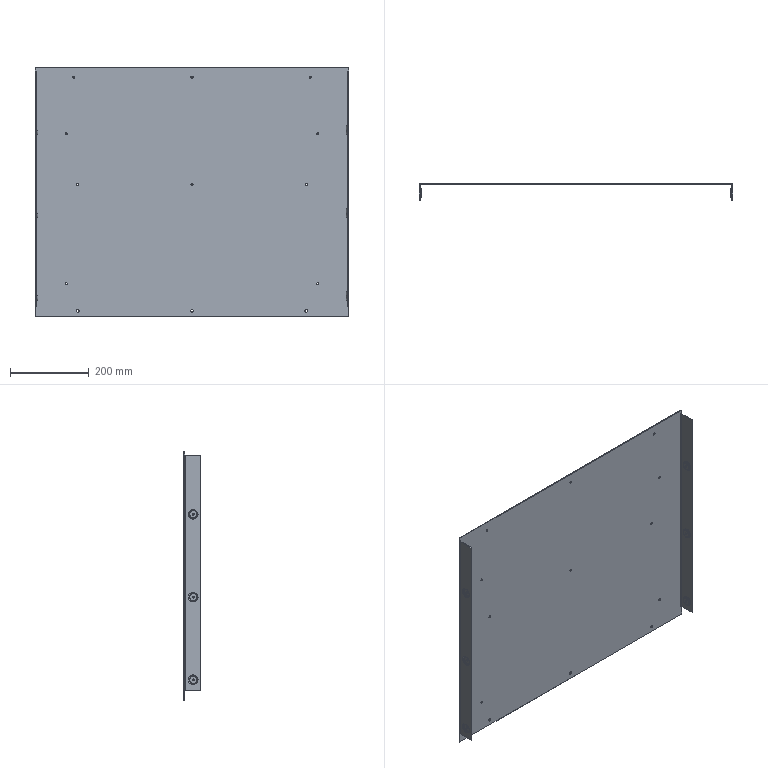Part | STEP file | 1 solid | 152 faces | box 795 x 42 x 633 mm | volume 1100610 mm3 | cylinder 66 | torus 48 | plane 38 | commonest cylinder face diameters 5.3 x20 4.7 x12 20 x12 24 x12 7 x8 3 x2